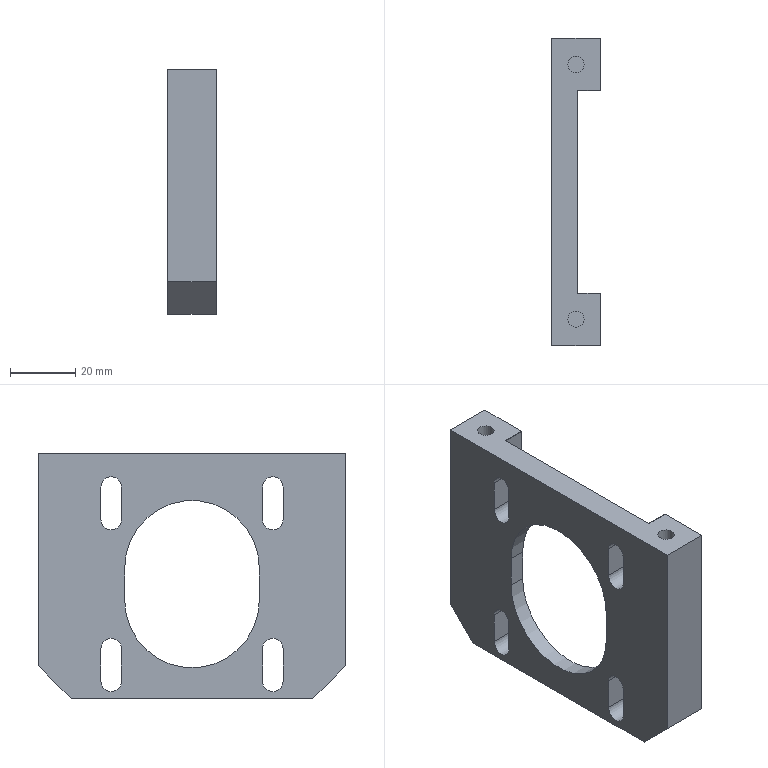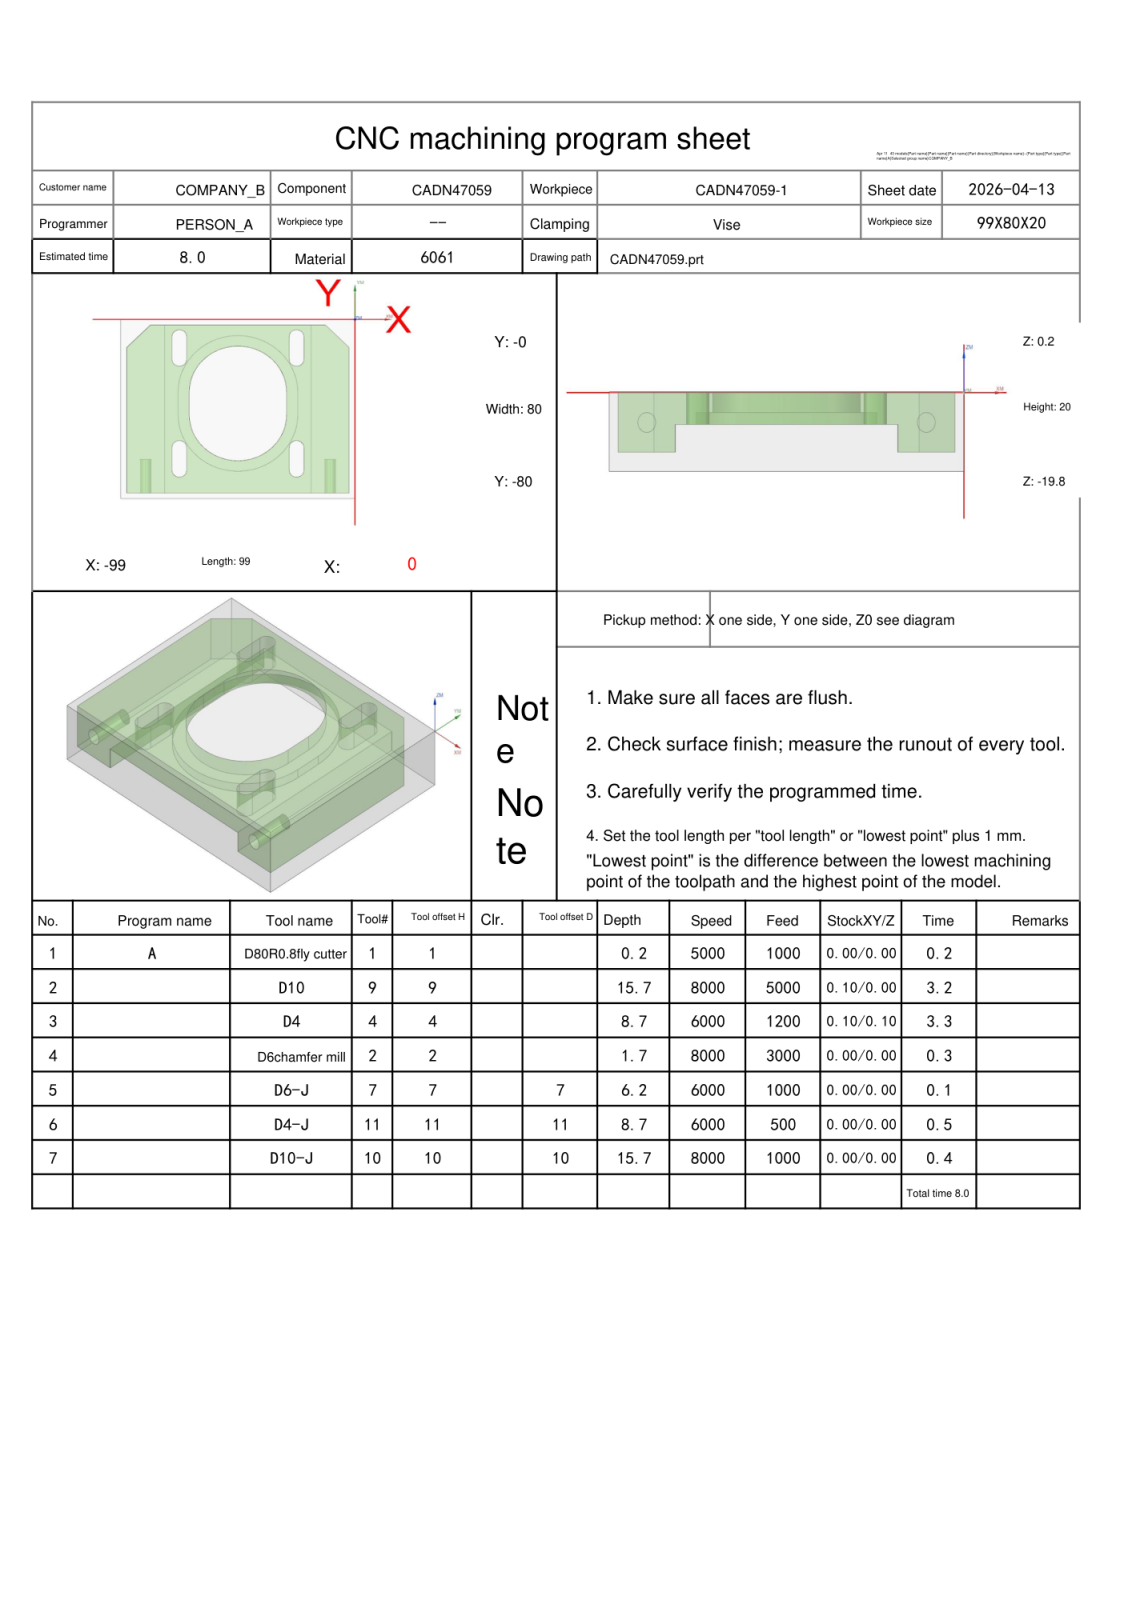NC program | NX | posted by the shop | part box 15 x 94 x 75 mm
Lines 1 to 937 of 2209:
%
O0001
(Machine time: 9.35 MIN)
(===Total Tool:7===)
(T1=D80R0.8 D=80.  R=0.8  D-  H01 Z=0.    )
(T9=D10     D=10.  R=0.   D-  H09 Z=-15.5 )
(T4=D4      D=4.   R=0.   D-  H04 Z=-8.5  )
(T2=D6chamfer mill   D=6.   R=0.   D-  H02 Z=-1.5  )
(T7=D6-J    D=6.   R=0.   D7  H07 Z=-6.   )
(T11=D4-J   D=4.   R=0.   D11 H11 Z=-8.5  )
(T10=D10-J  D=10.  R=0.   D10 H10 Z=-15.5 )
G80 G90 G17 G49 G40
G91 G28 Z0
M01
N1 T01 M06
(D80R0.8  D=80. R=0.8 H=01 ce=0.00 di=0.00)
G00 G90 G54 X-141.5 Y-40. M03 S5000
G43 H01 Z20.
M08
Z2.
G01 Z0.0 F1000.
X-136.5
X37.5
X42.5
Z2.
G00 Z20.
G91 G28 Z0.0
M05
M09
G91 G28 Z0.0
M01
N2 T09 M06
(D10  D=10. R=0. H=09 ce=0.10 di=0.00)
G00 G90 G54 X-49.5 Y-82.6 M03 S8000
G43 H09 Z20.
M08
Z.5
G01 X-96.5 Z.4 F5000.
G02 X-101.6 Y-77.5 Z.383 I0.0 J5.1
G01 Y-12.5 Z.245
G02 X-100.106 Y-8.894 Z.236 I5.1 J0.0
G01 X-90.106 Y1.106 Z.206
G02 X-86.5 Y2.6 Z.198 I3.606 J-3.606
G01 X-12.5 Z.04
G02 X-8.894 Y1.106 Z.032 I0.0 J-5.1
G01 X1.106 Y-8.894 Z.002
G02 X2.6 Y-12.5 Z-.007 I-3.606 J-3.606
G01 Y-77.5 Z-.145
G02 X-2.5 Y-82.6 Z-.162 I-5.1 J0.0
G01 X-96.5 Z-.362
G02 X-101.6 Y-77.5 Z-.379 I0.0 J5.1
G01 Y-12.5 Z-.517
G02 X-100.106 Y-8.894 Z-.526 I5.1 J0.0
G01 X-90.106 Y1.106 Z-.556
G02 X-86.5 Y2.6 Z-.564 I3.606 J-3.606
G01 X-12.5 Z-.722
G02 X-8.894 Y1.106 Z-.73 I0.0 J-5.1
G01 X1.106 Y-8.894 Z-.76
G02 X2.6 Y-12.5 Z-.769 I-3.606 J-3.606
G01 Y-77.5 Z-.907
G02 X-2.5 Y-82.6 Z-.924 I-5.1 J0.0
G01 X-96.5 Z-1.124
G02 X-101.6 Y-77.5 Z-1.141 I0.0 J5.1
G01 Y-12.5 Z-1.279
G02 X-100.106 Y-8.894 Z-1.288 I5.1 J0.0
G01 X-90.106 Y1.106 Z-1.318
G02 X-86.5 Y2.6 Z-1.326 I3.606 J-3.606
G01 X-12.5 Z-1.483
G02 X-8.894 Y1.106 Z-1.492 I0.0 J-5.1
G01 X1.106 Y-8.894 Z-1.522
G02 X2.6 Y-12.5 Z-1.531 I-3.606 J-3.606
G01 Y-77.5 Z-1.669
G02 X-2.5 Y-82.6 Z-1.686 I-5.1 J0.0
G01 X-96.5 Z-1.886
G02 X-101.6 Y-77.5 Z-1.903 I0.0 J5.1
G01 Y-12.5 Z-2.041
G02 X-100.106 Y-8.894 Z-2.049 I5.1 J0.0
G01 X-90.106 Y1.106 Z-2.079
G02 X-86.5 Y2.6 Z-2.088 I3.606 J-3.606
G01 X-12.5 Z-2.245
G02 X-8.894 Y1.106 Z-2.254 I0.0 J-5.1
G01 X1.106 Y-8.894 Z-2.284
G02 X2.6 Y-12.5 Z-2.292 I-3.606 J-3.606
G01 Y-77.5 Z-2.431
G02 X-2.5 Y-82.6 Z-2.448 I-5.1 J0.0
G01 X-96.5 Z-2.648
G02 X-101.6 Y-77.5 Z-2.665 I0.0 J5.1
G01 Y-12.5 Z-2.803
G02 X-100.106 Y-8.894 Z-2.811 I5.1 J0.0
G01 X-90.106 Y1.106 Z-2.841
G02 X-86.5 Y2.6 Z-2.85 I3.606 J-3.606
G01 X-12.5 Z-3.007
G02 X-8.894 Y1.106 Z-3.016 I0.0 J-5.1
G01 X1.106 Y-8.894 Z-3.046
G02 X2.6 Y-12.5 Z-3.054 I-3.606 J-3.606
G01 Y-77.5 Z-3.193
G02 X-2.5 Y-82.6 Z-3.21 I-5.1 J0.0
G01 X-96.5 Z-3.409
G02 X-101.6 Y-77.5 Z-3.426 I0.0 J5.1
G01 Y-12.5 Z-3.565
G02 X-100.106 Y-8.894 Z-3.573 I5.1 J0.0
G01 X-90.106 Y1.106 Z-3.603
G02 X-86.5 Y2.6 Z-3.612 I3.606 J-3.606
G01 X-12.5 Z-3.769
G02 X-8.894 Y1.106 Z-3.778 I0.0 J-5.1
G01 X1.106 Y-8.894 Z-3.808
G02 X2.6 Y-12.5 Z-3.816 I-3.606 J-3.606
G01 Y-77.5 Z-3.954
G02 X-2.5 Y-82.6 Z-3.971 I-5.1 J0.0
G01 X-96.5 Z-4.171
G02 X-101.6 Y-77.5 Z-4.188 I0.0 J5.1
G01 Y-12.5 Z-4.327
G02 X-100.106 Y-8.894 Z-4.335 I5.1 J0.0
G01 X-90.106 Y1.106 Z-4.365
G02 X-86.5 Y2.6 Z-4.374 I3.606 J-3.606
G01 X-12.5 Z-4.531
G02 X-8.894 Y1.106 Z-4.54 I0.0 J-5.1
G01 X1.106 Y-8.894 Z-4.57
G02 X2.6 Y-12.5 Z-4.578 I-3.606 J-3.606
G01 Y-77.5 Z-4.716
G02 X-2.5 Y-82.6 Z-4.733 I-5.1 J0.0
G01 X-96.5 Z-4.933
G02 X-101.6 Y-77.5 Z-4.95 I0.0 J5.1
G01 Y-12.5 Z-5.089
G02 X-100.106 Y-8.894 Z-5.097 I5.1 J0.0
G01 X-90.106 Y1.106 Z-5.127
G02 X-86.5 Y2.6 Z-5.136 I3.606 J-3.606
G01 X-12.5 Z-5.293
G02 X-8.894 Y1.106 Z-5.301 I0.0 J-5.1
G01 X1.106 Y-8.894 Z-5.332
G02 X2.6 Y-12.5 Z-5.34 I-3.606 J-3.606
G01 Y-77.5 Z-5.478
G02 X-2.5 Y-82.6 Z-5.495 I-5.1 J0.0
G01 X-96.5 Z-5.695
G02 X-101.6 Y-77.5 Z-5.712 I0.0 J5.1
G01 Y-12.5 Z-5.85
G02 X-100.106 Y-8.894 Z-5.859 I5.1 J0.0
G01 X-90.106 Y1.106 Z-5.889
G02 X-86.5 Y2.6 Z-5.898 I3.606 J-3.606
G01 X-12.5 Z-6.055
G02 X-8.894 Y1.106 Z-6.063 I0.0 J-5.1
G01 X1.106 Y-8.894 Z-6.093
G02 X2.6 Y-12.5 Z-6.102 I-3.606 J-3.606
G01 Y-77.5 Z-6.24
G02 X-2.5 Y-82.6 Z-6.257 I-5.1 J0.0
G01 X-96.5 Z-6.457
G02 X-101.6 Y-77.5 Z-6.474 I0.0 J5.1
G01 Y-12.5 Z-6.612
G02 X-100.106 Y-8.894 Z-6.621 I5.1 J0.0
G01 X-90.106 Y1.106 Z-6.651
G02 X-86.5 Y2.6 Z-6.659 I3.606 J-3.606
G01 X-12.5 Z-6.817
G02 X-8.894 Y1.106 Z-6.825 I0.0 J-5.1
G01 X1.106 Y-8.894 Z-6.855
G02 X2.6 Y-12.5 Z-6.864 I-3.606 J-3.606
G01 Y-77.5 Z-7.002
G02 X-2.5 Y-82.6 Z-7.019 I-5.1 J0.0
G01 X-96.5 Z-7.219
G02 X-101.6 Y-77.5 Z-7.236 I0.0 J5.1
G01 Y-12.5 Z-7.374
G02 X-100.106 Y-8.894 Z-7.383 I5.1 J0.0
G01 X-90.106 Y1.106 Z-7.413
G02 X-86.5 Y2.6 Z-7.421 I3.606 J-3.606
G01 X-12.5 Z-7.579
G02 X-8.894 Y1.106 Z-7.587 I0.0 J-5.1
G01 X1.106 Y-8.894 Z-7.617
G02 X2.6 Y-12.5 Z-7.626 I-3.606 J-3.606
G01 Y-77.5 Z-7.764
G02 X-2.5 Y-82.6 Z-7.781 I-5.1 J0.0
G01 X-96.5 Z-7.981
G02 X-101.6 Y-77.5 Z-7.998 I0.0 J5.1
G01 Y-12.5 Z-8.136
G02 X-100.106 Y-8.894 Z-8.145 I5.1 J0.0
G01 X-90.106 Y1.106 Z-8.175
G02 X-86.5 Y2.6 Z-8.183 I3.606 J-3.606
G01 X-12.5 Z-8.341
G02 X-8.894 Y1.106 Z-8.349 I0.0 J-5.1
G01 X1.106 Y-8.894 Z-8.379
G02 X2.6 Y-12.5 Z-8.388 I-3.606 J-3.606
G01 Y-77.5 Z-8.526
G02 X-2.5 Y-82.6 Z-8.543 I-5.1 J0.0
G01 X-96.5 Z-8.743
G02 X-101.6 Y-77.5 Z-8.76 I0.0 J5.1
G01 Y-12.5 Z-8.898
G02 X-100.106 Y-8.894 Z-8.907 I5.1 J0.0
G01 X-90.106 Y1.106 Z-8.937
G02 X-86.5 Y2.6 Z-8.945 I3.606 J-3.606
G01 X-12.5 Z-9.102
G02 X-8.894 Y1.106 Z-9.111 I0.0 J-5.1
G01 X1.106 Y-8.894 Z-9.141
G02 X2.6 Y-12.5 Z-9.15 I-3.606 J-3.606
G01 Y-77.5 Z-9.288
G02 X-2.5 Y-82.6 Z-9.305 I-5.1 J0.0
G01 X-96.5 Z-9.505
G02 X-101.6 Y-77.5 Z-9.522 I0.0 J5.1
G01 Y-12.5 Z-9.66
G02 X-100.106 Y-8.894 Z-9.668 I5.1 J0.0
G01 X-90.106 Y1.106 Z-9.699
G02 X-86.5 Y2.6 Z-9.707 I3.606 J-3.606
G01 X-12.5 Z-9.864
G02 X-8.894 Y1.106 Z-9.873 I0.0 J-5.1
G01 X1.106 Y-8.894 Z-9.903
G02 X2.6 Y-12.5 Z-9.911 I-3.606 J-3.606
G01 Y-77.5 Z-10.05
G02 X-2.5 Y-82.6 Z-10.067 I-5.1 J0.0
G01 X-96.5 Z-10.267
G02 X-101.6 Y-77.5 Z-10.284 I0.0 J5.1
G01 Y-12.5 Z-10.422
G02 X-100.106 Y-8.894 Z-10.43 I5.1 J0.0
G01 X-90.106 Y1.106 Z-10.46
G02 X-86.5 Y2.6 Z-10.469 I3.606 J-3.606
G01 X-12.5 Z-10.626
G02 X-8.894 Y1.106 Z-10.635 I0.0 J-5.1
G01 X1.106 Y-8.894 Z-10.665
G02 X2.6 Y-12.5 Z-10.673 I-3.606 J-3.606
G01 Y-77.5 Z-10.812
G02 X-2.5 Y-82.6 Z-10.829 I-5.1 J0.0
G01 X-96.5 Z-11.029
G02 X-101.6 Y-77.5 Z-11.046 I0.0 J5.1
G01 Y-12.5 Z-11.184
G02 X-100.106 Y-8.894 Z-11.192 I5.1 J0.0
G01 X-90.106 Y1.106 Z-11.222
G02 X-86.5 Y2.6 Z-11.231 I3.606 J-3.606
G01 X-12.5 Z-11.388
G02 X-8.894 Y1.106 Z-11.397 I0.0 J-5.1
G01 X1.106 Y-8.894 Z-11.427
G02 X2.6 Y-12.5 Z-11.435 I-3.606 J-3.606
G01 Y-77.5 Z-11.574
G02 X-2.5 Y-82.6 Z-11.591 I-5.1 J0.0
G01 X-96.5 Z-11.79
G02 X-101.6 Y-77.5 Z-11.807 I0.0 J5.1
G01 Y-12.5 Z-11.946
G02 X-100.106 Y-8.894 Z-11.954 I5.1 J0.0
G01 X-90.106 Y1.106 Z-11.984
G02 X-86.5 Y2.6 Z-11.993 I3.606 J-3.606
G01 X-12.5 Z-12.15
G02 X-8.894 Y1.106 Z-12.159 I0.0 J-5.1
G01 X1.106 Y-8.894 Z-12.189
G02 X2.6 Y-12.5 Z-12.197 I-3.606 J-3.606
G01 Y-77.5 Z-12.335
G02 X-2.5 Y-82.6 Z-12.352 I-5.1 J0.0
G01 X-96.5 Z-12.552
G02 X-101.6 Y-77.5 Z-12.569 I0.0 J5.1
G01 Y-12.5 Z-12.708
G02 X-100.106 Y-8.894 Z-12.716 I5.1 J0.0
G01 X-90.106 Y1.106 Z-12.746
G02 X-86.5 Y2.6 Z-12.755 I3.606 J-3.606
G01 X-12.5 Z-12.912
G02 X-8.894 Y1.106 Z-12.921 I0.0 J-5.1
G01 X1.106 Y-8.894 Z-12.951
G02 X2.6 Y-12.5 Z-12.959 I-3.606 J-3.606
G01 Y-77.5 Z-13.097
G02 X-2.5 Y-82.6 Z-13.114 I-5.1 J0.0
G01 X-96.5 Z-13.314
G02 X-101.6 Y-77.5 Z-13.331 I0.0 J5.1
G01 Y-12.5 Z-13.469
G02 X-100.106 Y-8.894 Z-13.478 I5.1 J0.0
G01 X-90.106 Y1.106 Z-13.508
G02 X-86.5 Y2.6 Z-13.517 I3.606 J-3.606
G01 X-12.5 Z-13.674
G02 X-8.894 Y1.106 Z-13.682 I0.0 J-5.1
G01 X1.106 Y-8.894 Z-13.712
G02 X2.6 Y-12.5 Z-13.721 I-3.606 J-3.606
G01 Y-77.5 Z-13.859
G02 X-2.5 Y-82.6 Z-13.876 I-5.1 J0.0
G01 X-96.5 Z-14.076
G02 X-101.6 Y-77.5 Z-14.093 I0.0 J5.1
G01 Y-12.5 Z-14.231
G02 X-100.106 Y-8.894 Z-14.24 I5.1 J0.0
G01 X-90.106 Y1.106 Z-14.27
G02 X-86.5 Y2.6 Z-14.278 I3.606 J-3.606
G01 X-12.5 Z-14.436
G02 X-8.894 Y1.106 Z-14.444 I0.0 J-5.1
G01 X1.106 Y-8.894 Z-14.474
G02 X2.6 Y-12.5 Z-14.483 I-3.606 J-3.606
G01 Y-77.5 Z-14.621
G02 X-2.5 Y-82.6 Z-14.638 I-5.1 J0.0
G01 X-96.5 Z-14.838
G02 X-101.6 Y-77.5 Z-14.855 I0.0 J5.1
G01 Y-12.5 Z-14.993
G02 X-100.106 Y-8.894 Z-15.002 I5.1 J0.0
G01 X-90.106 Y1.106 Z-15.032
G02 X-86.5 Y2.6 Z-15.04 I3.606 J-3.606
G01 X-12.5 Z-15.198
G02 X-8.894 Y1.106 Z-15.206 I0.0 J-5.1
G01 X1.106 Y-8.894 Z-15.236
G02 X2.6 Y-12.5 Z-15.245 I-3.606 J-3.606
G01 Y-77.5 Z-15.383
G02 X-2.5 Y-82.6 Z-15.4 I-5.1 J0.0
G01 X-49.5 Z-15.5
X-96.5
G02 X-101.6 Y-77.5 I0.0 J5.1
G01 Y-12.5
G02 X-100.106 Y-8.894 I5.1 J0.0
G01 X-90.106 Y1.106
G02 X-86.5 Y2.6 I3.606 J-3.606
G01 X-12.5
G02 X-8.894 Y1.106 I0.0 J-5.1
G01 X1.106 Y-8.894
G02 X2.6 Y-12.5 I-3.606 J-3.606
G01 Y-77.5
G02 X-2.5 Y-82.6 I-5.1 J0.0
G01 X-49.5
X-50.
Z-14.5
G00 Z20.
G00 G90 X-55.245 Y-38.997 M03 S8000
Z10.2
Z1.5
G02 X-55.245 Y-38.997 Z.018 I-4.255 J1.466 F3000.
X-63.182 Y-40.118 Z-.5 I-4.255 J1.466
G01 X-65. Y-37.531
Y-32.5
G02 X-49.5 Y-17. I15.5 J0.0
X-34. Y-32.5 I0.0 J-15.5
G01 Y-42.5
G02 X-49.5 Y-58. I-15.5 J0.0
X-64.999 Y-42.703 I0.0 J15.5
G01 X-65. Y-37.531
Y-33.25
G02 X-64.318 Y-32.303 I1. J0.0
G01 X-58.118 Y-30.225
G03 X-57.496 Y-29.616 I-.318 J.948
G02 X-49.5 Y-24. I7.996 J-2.884
X-41. Y-32.5 I0.0 J-8.5
G01 Y-42.5
G02 X-49.5 Y-51. I-8.5 J0.0
X-57.999 Y-42.649 I0.0 J8.5
G01 X-58. Y-37.531
Y-35.733
G02 X-57.34 Y-34.793 I1. J0.0
G01 X-51.547 Y-32.698
G03 X-50.932 Y-32.055 I-.34 J.94
G02 X-49.5 Y-31. I1.432 J-.445
X-48. Y-32.5 I0.0 J-1.5
G01 Y-42.5
G02 X-49.5 Y-44. I-1.5 J0.0
X-50.999 Y-42.562 I0.0 J1.5
G01 X-51. Y-37.625
Y-32.531
Y-32.5
G02 X-50.927 Y-32.039 I1.5 J0.0
G03 X-50.588 Y-29.886 I-6.661 J2.153
X-55.435 Y-23.225 I-7. J0.0
G01 Z.7
G00 Z3.
G01 X-55.245 Y-38.997 F6000.
G00 Z1.
G02 X-55.245 Y-38.997 Z-.482 I-4.255 J1.466 F3000.
X-63.182 Y-40.118 Z-1. I-4.255 J1.466
G01 X-65. Y-37.531
Y-32.5
G02 X-49.5 Y-17. I15.5 J0.0
X-34. Y-32.5 I0.0 J-15.5
G01 Y-42.5
G02 X-49.5 Y-58. I-15.5 J0.0
X-64.999 Y-42.703 I0.0 J15.5
G01 X-65. Y-37.531
Y-32.531
G02 X-64.221 Y-31.556 I1. J0.0
G01 X-58.193 Y-30.19
G03 X-57.476 Y-29.561 I-.221 J.975
G02 X-49.5 Y-24. I7.976 J-2.939
X-41. Y-32.5 I0.0 J-8.5
G01 Y-42.5
G02 X-49.5 Y-51. I-8.5 J0.0
X-57.999 Y-42.649 I0.0 J8.5
G01 X-58. Y-37.531
Y-35.655
G02 X-57.44 Y-34.757 I1. J0.0
G01 X-50.515 Y-31.365
X-50.373 Y-31.28
G02 X-49.5 Y-31. I.873 J-1.22
X-48. Y-32.5 I0.0 J-1.5
G01 Y-42.5
G02 X-49.5 Y-44. I-1.5 J0.0
X-50.999 Y-42.562 I0.0 J1.5
G01 X-51. Y-37.625
Y-32.531
Y-32.5
G02 X-50.927 Y-32.039 I1.5 J0.0
G03 X-50.588 Y-29.886 I-6.661 J2.153
X-55.435 Y-23.225 I-7. J0.0
G01 Z.2
G00 Z2.5
G01 X-55.245 Y-38.997 F6000.
G00 Z.5
G02 X-55.245 Y-38.997 Z-.982 I-4.255 J1.466 F3000.
X-63.182 Y-40.118 Z-1.5 I-4.255 J1.466
G01 X-65. Y-37.531
Y-32.5
G02 X-49.5 Y-17. I15.5 J0.0
X-34. Y-32.5 I0.0 J-15.5
G01 Y-42.5
G02 X-49.5 Y-58. I-15.5 J0.0
X-64.999 Y-42.703 I0.0 J15.5
G01 X-65. Y-37.531
Y-32.531
G02 X-64.221 Y-31.556 I1. J0.0
G01 X-58.193 Y-30.19
G03 X-57.476 Y-29.561 I-.221 J.975
G02 X-49.5 Y-24. I7.976 J-2.939
X-41. Y-32.5 I0.0 J-8.5
G01 Y-42.5
G02 X-49.5 Y-51. I-8.5 J0.0
X-57.999 Y-42.649 I0.0 J8.5
G01 X-58. Y-37.531
Y-35.733
G02 X-57.34 Y-34.793 I1. J0.0
G01 X-51.547 Y-32.698
G03 X-50.932 Y-32.055 I-.34 J.94
G02 X-49.5 Y-31. I1.432 J-.445
X-48. Y-32.5 I0.0 J-1.5
G01 Y-42.5
G02 X-49.5 Y-44. I-1.5 J0.0
X-50.999 Y-42.562 I0.0 J1.5
G01 X-51. Y-37.625
Y-32.531
Y-32.5
G02 X-50.927 Y-32.039 I1.5 J0.0
G03 X-50.588 Y-29.886 I-6.661 J2.153
X-55.435 Y-23.225 I-7. J0.0
G01 Z-.3
G00 Z2.
G01 X-55.245 Y-38.997 F6000.
G00 Z0.0
G02 X-55.245 Y-38.997 Z-1.482 I-4.255 J1.466 F3000.
X-63.182 Y-40.118 Z-2. I-4.255 J1.466
G01 X-65. Y-37.531
Y-32.5
G02 X-49.5 Y-17. I15.5 J0.0
X-34. Y-32.5 I0.0 J-15.5
G01 Y-42.5
G02 X-49.5 Y-58. I-15.5 J0.0
X-64.999 Y-42.703 I0.0 J15.5
G01 X-65. Y-37.531
Y-32.531
G02 X-64.221 Y-31.556 I1. J0.0
G01 X-58.193 Y-30.19
G03 X-57.476 Y-29.561 I-.221 J.975
G02 X-49.5 Y-24. I7.976 J-2.939
X-41. Y-32.5 I0.0 J-8.5
G01 Y-42.5
G02 X-49.5 Y-51. I-8.5 J0.0
X-57.999 Y-42.649 I0.0 J8.5
G01 X-58. Y-37.531
Y-35.733
G02 X-57.34 Y-34.793 I1. J0.0
G01 X-51.547 Y-32.698
G03 X-50.932 Y-32.055 I-.34 J.94
G02 X-49.5 Y-31. I1.432 J-.445
X-48. Y-32.5 I0.0 J-1.5
G01 Y-42.5
G02 X-49.5 Y-44. I-1.5 J0.0
X-50.999 Y-42.562 I0.0 J1.5
G01 X-51. Y-37.625
Y-32.531
Y-32.5
G02 X-50.927 Y-32.039 I1.5 J0.0
G03 X-50.588 Y-29.886 I-6.661 J2.153
X-55.435 Y-23.225 I-7. J0.0
G01 Z-.8
G00 Z1.5
G01 X-55.245 Y-38.997 F6000.
G00 Z-.5
G02 X-55.245 Y-38.997 Z-1.982 I-4.255 J1.466 F3000.
X-63.182 Y-40.118 Z-2.5 I-4.255 J1.466
G01 X-65. Y-37.531
Y-32.5
G02 X-49.5 Y-17. I15.5 J0.0
X-34. Y-32.5 I0.0 J-15.5
G01 Y-42.5
G02 X-49.5 Y-58. I-15.5 J0.0
X-64.999 Y-42.703 I0.0 J15.5
G01 X-65. Y-37.531
Y-32.531
G02 X-64.221 Y-31.556 I1. J0.0
G01 X-58.193 Y-30.19
G03 X-57.476 Y-29.561 I-.221 J.975
G02 X-49.5 Y-24. I7.976 J-2.939
X-41. Y-32.5 I0.0 J-8.5
G01 Y-42.5
G02 X-49.5 Y-51. I-8.5 J0.0
X-57.999 Y-42.649 I0.0 J8.5
G01 X-58. Y-37.531
Y-35.733
G02 X-57.34 Y-34.793 I1. J0.0
G01 X-51.547 Y-32.698
G03 X-50.932 Y-32.055 I-.34 J.94
G02 X-49.5 Y-31. I1.432 J-.445
X-48. Y-32.5 I0.0 J-1.5
G01 Y-42.5
G02 X-49.5 Y-44. I-1.5 J0.0
X-50.999 Y-42.562 I0.0 J1.5
G01 X-51. Y-37.625
Y-32.531
Y-32.5
G02 X-50.927 Y-32.039 I1.5 J0.0
G03 X-50.588 Y-29.886 I-6.661 J2.153
X-55.435 Y-23.225 I-7. J0.0
G01 Z-1.3
G00 Z1.
G01 X-55.245 Y-38.997 F6000.
G00 Z-1.
G02 X-55.245 Y-38.997 Z-2.482 I-4.255 J1.466 F3000.
X-63.182 Y-40.118 Z-3. I-4.255 J1.466
G01 X-65. Y-37.531
Y-32.5
G02 X-49.5 Y-17. I15.5 J0.0
X-34. Y-32.5 I0.0 J-15.5
G01 Y-42.5
G02 X-49.5 Y-58. I-15.5 J0.0
X-64.999 Y-42.703 I0.0 J15.5
G01 X-65. Y-37.531
Y-32.531
G02 X-64.221 Y-31.556 I1. J0.0
G01 X-58.193 Y-30.19
G03 X-57.476 Y-29.561 I-.221 J.975
G02 X-49.5 Y-24. I7.976 J-2.939
X-41. Y-32.5 I0.0 J-8.5
G01 Y-42.5
G02 X-49.5 Y-51. I-8.5 J0.0
X-57.999 Y-42.649 I0.0 J8.5
G01 X-58. Y-37.531
Y-35.733
G02 X-57.34 Y-34.793 I1. J0.0
G01 X-51.547 Y-32.698
G03 X-50.932 Y-32.055 I-.34 J.94
G02 X-49.5 Y-31. I1.432 J-.445
X-48. Y-32.5 I0.0 J-1.5
G01 Y-42.5
G02 X-49.5 Y-44. I-1.5 J0.0
X-50.999 Y-42.562 I0.0 J1.5
G01 X-51. Y-37.625
Y-32.531
Y-32.5
G02 X-50.927 Y-32.039 I1.5 J0.0
G03 X-50.588 Y-29.886 I-6.661 J2.153
X-55.435 Y-23.225 I-7. J0.0
G01 Z-1.8
G00 Z.5
G01 X-55.245 Y-38.997 F6000.
G00 Z-1.5
G02 X-55.245 Y-38.997 Z-2.982 I-4.255 J1.466 F3000.
X-63.182 Y-40.118 Z-3.5 I-4.255 J1.466
G01 X-65. Y-37.531
Y-32.5
G02 X-49.5 Y-17. I15.5 J0.0
X-34. Y-32.5 I0.0 J-15.5
G01 Y-42.5
G02 X-49.5 Y-58. I-15.5 J0.0
X-64.999 Y-42.703 I0.0 J15.5
G01 X-65. Y-37.531
Y-33.25
G02 X-64.318 Y-32.303 I1. J0.0
G01 X-58.118 Y-30.225
G03 X-57.496 Y-29.616 I-.318 J.948
G02 X-49.5 Y-24. I7.996 J-2.884
X-41. Y-32.5 I0.0 J-8.5
G01 Y-42.5
G02 X-49.5 Y-51. I-8.5 J0.0
X-57.999 Y-42.649 I0.0 J8.5
G01 X-58. Y-37.531
Y-35.733
G02 X-57.34 Y-34.793 I1. J0.0
G01 X-51.547 Y-32.698
G03 X-50.932 Y-32.055 I-.34 J.94
G02 X-49.5 Y-31. I1.432 J-.445
X-48. Y-32.5 I0.0 J-1.5
G01 Y-42.5
G02 X-49.5 Y-44. I-1.5 J0.0
X-50.999 Y-42.562 I0.0 J1.5
G01 X-51. Y-37.625
Y-32.531
Y-32.5
G02 X-50.927 Y-32.039 I1.5 J0.0
G03 X-50.588 Y-29.886 I-6.661 J2.153
X-55.435 Y-23.225 I-7. J0.0
G01 Z-2.3
G00 Z0.0
G01 X-55.245 Y-38.997 F6000.
G00 Z-2.
G02 X-55.245 Y-38.997 Z-3.482 I-4.255 J1.466 F3000.
X-63.182 Y-40.118 Z-4. I-4.255 J1.466
G01 X-65. Y-37.531
Y-32.5
G02 X-49.5 Y-17. I15.5 J0.0
X-34. Y-32.5 I0.0 J-15.5
G01 Y-42.5
G02 X-49.5 Y-58. I-15.5 J0.0
X-64.999 Y-42.703 I0.0 J15.5
G01 X-65. Y-37.531
Y-32.531
G02 X-64.221 Y-31.556 I1. J0.0
G01 X-58.193 Y-30.19
G03 X-57.476 Y-29.561 I-.221 J.975
G02 X-49.5 Y-24. I7.976 J-2.939
X-41. Y-32.5 I0.0 J-8.5
G01 Y-42.5
G02 X-49.5 Y-51. I-8.5 J0.0
X-57.999 Y-42.649 I0.0 J8.5
G01 X-58. Y-37.531
Y-35.733
G02 X-57.34 Y-34.793 I1. J0.0
G01 X-51.547 Y-32.698
G03 X-50.932 Y-32.055 I-.34 J.94
G02 X-49.5 Y-31. I1.432 J-.445
X-48. Y-32.5 I0.0 J-1.5
G01 Y-42.5
G02 X-49.5 Y-44. I-1.5 J0.0
X-50.999 Y-42.562 I0.0 J1.5
G01 X-51. Y-37.626
Y-32.531
Y-32.5
G02 X-50.927 Y-32.039 I1.5 J0.0
G03 X-50.588 Y-29.886 I-6.661 J2.153
X-55.435 Y-23.225 I-7. J0.0
G01 Z-2.8
G00 Z-.5
G01 X-55.245 Y-38.997 F6000.
G00 Z-2.5
G02 X-55.245 Y-38.997 Z-3.982 I-4.255 J1.466 F3000.
X-63.182 Y-40.118 Z-4.5 I-4.255 J1.466
G01 X-65. Y-37.531
Y-32.5
G02 X-49.5 Y-17. I15.5 J0.0
X-34. Y-32.5 I0.0 J-15.5
G01 Y-42.5
G02 X-49.5 Y-58. I-15.5 J0.0
X-64.999 Y-42.703 I0.0 J15.5
G01 X-65. Y-37.531
Y-33.25
G02 X-64.318 Y-32.303 I1. J0.0
G01 X-58.118 Y-30.225
G03 X-57.496 Y-29.616 I-.318 J.948
G02 X-49.5 Y-24. I7.996 J-2.884
X-41. Y-32.5 I0.0 J-8.5
G01 Y-42.5
G02 X-49.5 Y-51. I-8.5 J0.0
X-57.999 Y-42.649 I0.0 J8.5
G01 X-58. Y-37.531
Y-35.733
G02 X-57.34 Y-34.793 I1. J0.0
G01 X-51.547 Y-32.698
G03 X-50.932 Y-32.055 I-.34 J.94
G02 X-49.5 Y-31. I1.432 J-.445
X-48. Y-32.5 I0.0 J-1.5
G01 Y-42.5
G02 X-49.5 Y-44. I-1.5 J0.0
X-50.998 Y-42.577 I0.0 J1.5
G01 X-51. Y-32.53
Y-32.5
G02 X-50.927 Y-32.037 I1.5 J0.0
G03 X-50.586 Y-29.878 I-6.659 J2.159
X-55.427 Y-23.22 I-7. J0.0
G01 Z-3.3
G00 Z-1.
G01 X-55.245 Y-38.997 F6000.
G00 Z-3.
G02 X-55.245 Y-38.997 Z-4.482 I-4.255 J1.466 F3000.
X-63.182 Y-40.118 Z-5. I-4.255 J1.466
G01 X-65. Y-37.531
Y-32.5
G02 X-49.5 Y-17. I15.5 J0.0
X-34. Y-32.5 I0.0 J-15.5
G01 Y-42.5
G02 X-49.5 Y-58. I-15.5 J0.0
X-64.999 Y-42.703 I0.0 J15.5
G01 X-65. Y-37.531
Y-32.531
G02 X-64.221 Y-31.556 I1. J0.0
G01 X-58.193 Y-30.19
G03 X-57.476 Y-29.561 I-.221 J.975
G02 X-49.5 Y-24. I7.976 J-2.939
X-41. Y-32.5 I0.0 J-8.5
G01 Y-42.5
G02 X-49.5 Y-51. I-8.5 J0.0
X-57.999 Y-42.649 I0.0 J8.5
G01 X-58. Y-37.531
Y-35.733
G02 X-57.34 Y-34.793 I1. J0.0
G01 X-51.547 Y-32.698
G03 X-50.932 Y-32.055 I-.34 J.94
G02 X-49.5 Y-31. I1.432 J-.445
X-48. Y-32.5 I0.0 J-1.5
G01 Y-42.5
G02 X-49.5 Y-44. I-1.5 J0.0
X-50.999 Y-42.562 I0.0 J1.5
G01 X-51. Y-37.626
Y-32.531
Y-32.5
G02 X-50.927 Y-32.039 I1.5 J0.0
G03 X-50.588 Y-29.886 I-6.661 J2.153
X-55.435 Y-23.225 I-7. J0.0
G01 Z-3.8
G00 Z-1.5
G01 X-55.245 Y-38.997 F6000.
G00 Z-3.5
G02 X-55.245 Y-38.997 Z-4.982 I-4.255 J1.466 F3000.
X-63.182 Y-40.118 Z-5.5 I-4.255 J1.466
G01 X-65. Y-37.531
Y-32.5
G02 X-49.5 Y-17. I15.5 J0.0
X-34. Y-32.5 I0.0 J-15.5
G01 Y-42.5
G02 X-49.5 Y-58. I-15.5 J0.0
X-64.999 Y-42.703 I0.0 J15.5
G01 X-65. Y-37.531
Y-32.531
G02 X-64.221 Y-31.556 I1. J0.0
G01 X-58.193 Y-30.19
G03 X-57.476 Y-29.561 I-.221 J.975
G02 X-49.5 Y-24. I7.976 J-2.939
X-41. Y-32.5 I0.0 J-8.5
G01 Y-42.5
G02 X-49.5 Y-51. I-8.5 J0.0
X-57.999 Y-42.649 I0.0 J8.5
G01 X-58. Y-37.531
Y-35.733
G02 X-57.34 Y-34.793 I1. J0.0
G01 X-51.547 Y-32.698
G03 X-50.932 Y-32.055 I-.34 J.94
G02 X-49.5 Y-31. I1.432 J-.445
X-48. Y-32.5 I0.0 J-1.5
G01 Y-42.5
G02 X-49.5 Y-44. I-1.5 J0.0
X-50.999 Y-42.562 I0.0 J1.5
G01 X-51. Y-37.626
Y-32.531
Y-32.5
G02 X-50.927 Y-32.039 I1.5 J0.0
G03 X-50.588 Y-29.886 I-6.661 J2.153
X-55.435 Y-23.225 I-7. J0.0
G01 Z-4.3
G00 Z-2.
G01 X-55.245 Y-38.997 F6000.
G00 Z-4.
G02 X-55.245 Y-38.997 Z-5.482 I-4.255 J1.466 F3000.
X-63.182 Y-40.118 Z-6. I-4.255 J1.466
G01 X-65. Y-37.531
Y-32.5
G02 X-49.5 Y-17. I15.5 J0.0
X-34. Y-32.5 I0.0 J-15.5
G01 Y-42.5
G02 X-49.5 Y-58. I-15.5 J0.0
X-64.999 Y-42.703 I0.0 J15.5
G01 X-65. Y-37.531
Y-32.531
G02 X-64.221 Y-31.556 I1. J0.0
G01 X-58.193 Y-30.19
G03 X-57.476 Y-29.561 I-.221 J.975
G02 X-49.5 Y-24. I7.976 J-2.939
X-41. Y-32.5 I0.0 J-8.5
G01 Y-42.5
G02 X-49.5 Y-51. I-8.5 J0.0
X-57.999 Y-42.649 I0.0 J8.5
G01 X-58. Y-37.531
Y-35.733
G02 X-57.34 Y-34.793 I1. J0.0
G01 X-51.547 Y-32.698
G03 X-50.932 Y-32.055 I-.34 J.94
G02 X-49.5 Y-31. I1.432 J-.445
X-48. Y-32.5 I0.0 J-1.5
G01 Y-42.5
G02 X-49.5 Y-44. I-1.5 J0.0
X-50.999 Y-42.562 I0.0 J1.5
G01 X-51. Y-37.626
Y-32.531
Y-32.5
G02 X-50.927 Y-32.039 I1.5 J0.0
G03 X-50.588 Y-29.886 I-6.661 J2.153
X-55.435 Y-23.225 I-7. J0.0
G01 Z-4.8
G00 Z-2.5
G01 X-55.245 Y-38.997 F6000.
G00 Z-4.5
G02 X-55.245 Y-38.997 Z-5.982 I-4.255 J1.466 F3000.
X-63.182 Y-40.118 Z-6.5 I-4.255 J1.466
G01 X-65. Y-37.531
Y-32.5
G02 X-49.5 Y-17. I15.5 J0.0
X-34. Y-32.5 I0.0 J-15.5
G01 Y-42.5
G02 X-49.5 Y-58. I-15.5 J0.0
X-64.999 Y-42.703 I0.0 J15.5
G01 X-65. Y-37.531
Y-32.531
G02 X-64.221 Y-31.556 I1. J0.0
G01 X-58.193 Y-30.19
G03 X-57.476 Y-29.561 I-.221 J.975
G02 X-49.5 Y-24. I7.976 J-2.939
X-41. Y-32.5 I0.0 J-8.5
G01 Y-42.5
G02 X-49.5 Y-51. I-8.5 J0.0
X-57.999 Y-42.649 I0.0 J8.5
G01 X-58. Y-37.531
Y-35.733
G02 X-57.34 Y-34.793 I1. J0.0
G01 X-51.547 Y-32.698
G03 X-50.932 Y-32.055 I-.34 J.94
G02 X-49.5 Y-31. I1.432 J-.445
X-48. Y-32.5 I0.0 J-1.5
G01 Y-42.5
G02 X-49.5 Y-44. I-1.5 J0.0
X-50.999 Y-42.562 I0.0 J1.5
G01 X-51. Y-37.626
Y-32.531
Y-32.5
G02 X-50.927 Y-32.039 I1.5 J0.0
G03 X-50.588 Y-29.886 I-6.661 J2.153
X-55.435 Y-23.225 I-7. J0.0
G01 Z-5.3
G00 Z-3.
G01 X-55.245 Y-38.997 F6000.
G00 Z-5.
G02 X-55.245 Y-38.997 Z-6.482 I-4.255 J1.466 F3000.
X-63.182 Y-40.118 Z-7. I-4.255 J1.466
G01 X-65. Y-37.531
Y-32.5
G02 X-49.5 Y-17. I15.5 J0.0
X-34. Y-32.5 I0.0 J-15.5
G01 Y-42.5
G02 X-49.5 Y-58. I-15.5 J0.0
X-64.999 Y-42.703 I0.0 J15.5
G01 X-65. Y-37.531
Y-32.531
G02 X-64.221 Y-31.556 I1. J0.0
G01 X-58.193 Y-30.19
G03 X-57.476 Y-29.561 I-.221 J.975
G02 X-49.5 Y-24. I7.976 J-2.939
X-41. Y-32.5 I0.0 J-8.5
G01 Y-42.5
G02 X-49.5 Y-51. I-8.5 J0.0
X-57.999 Y-42.649 I0.0 J8.5
G01 X-58. Y-37.531
Y-35.733
G02 X-57.34 Y-34.793 I1. J0.0
G01 X-51.547 Y-32.698
G03 X-50.932 Y-32.055 I-.34 J.94
G02 X-49.5 Y-31. I1.432 J-.445
X-48. Y-32.5 I0.0 J-1.5
G01 Y-42.5
G02 X-49.5 Y-44. I-1.5 J0.0
X-50.999 Y-42.562 I0.0 J1.5
G01 X-51. Y-37.626
Y-32.531
Y-32.5
G02 X-50.927 Y-32.039 I1.5 J0.0
G03 X-50.588 Y-29.886 I-6.661 J2.153
X-55.435 Y-23.225 I-7. J0.0
G01 Z-5.8
G00 Z-3.5
G01 X-55.245 Y-38.997 F6000.
G00 Z-5.5
G02 X-55.245 Y-38.997 Z-6.982 I-4.255 J1.466 F3000.
X-63.182 Y-40.118 Z-7.5 I-4.255 J1.466
G01 X-65. Y-37.531
Y-32.5
G02 X-49.5 Y-17. I15.5 J0.0
X-34. Y-32.5 I0.0 J-15.5
G01 Y-42.5
G02 X-49.5 Y-58. I-15.5 J0.0
X-64.999 Y-42.703 I0.0 J15.5
G01 X-65. Y-37.531
Y-32.531
G02 X-64.221 Y-31.556 I1. J0.0
G01 X-58.193 Y-30.19
G03 X-57.476 Y-29.561 I-.221 J.975
G02 X-49.5 Y-24. I7.976 J-2.939
X-41. Y-32.5 I0.0 J-8.5
G01 Y-42.5
G02 X-49.5 Y-51. I-8.5 J0.0
X-57.999 Y-42.649 I0.0 J8.5
G01 X-58. Y-37.531
Y-35.733
G02 X-57.34 Y-34.793 I1. J0.0
G01 X-51.547 Y-32.698
G03 X-50.932 Y-32.055 I-.34 J.94
G02 X-49.5 Y-31. I1.432 J-.445
X-48. Y-32.5 I0.0 J-1.5
G01 Y-42.5
G02 X-49.5 Y-44. I-1.5 J0.0
X-50.999 Y-42.562 I0.0 J1.5
G01 X-51. Y-37.626
Y-32.531
Y-32.5
G02 X-50.927 Y-32.039 I1.5 J0.0
G03 X-50.588 Y-29.886 I-6.661 J2.153
X-55.435 Y-23.225 I-7. J0.0
G01 Z-6.3
G00 Z-4.
G01 X-55.245 Y-38.997 F6000.
G00 Z-6.
G02 X-55.245 Y-38.997 Z-7.482 I-4.255 J1.466 F3000.
X-63.182 Y-40.118 Z-8. I-4.255 J1.466
G01 X-65. Y-37.531
Y-32.5
G02 X-49.5 Y-17. I15.5 J0.0
X-34. Y-32.5 I0.0 J-15.5
G01 Y-42.5
G02 X-49.5 Y-58. I-15.5 J0.0
X-64.999 Y-42.703 I0.0 J15.5
G01 X-65. Y-37.531
Y-32.531
G02 X-64.221 Y-31.556 I1. J0.0
G01 X-58.193 Y-30.19
G03 X-57.476 Y-29.561 I-.221 J.975
G02 X-49.5 Y-24. I7.976 J-2.939
X-41. Y-32.5 I0.0 J-8.5
G01 Y-42.5
G02 X-49.5 Y-51. I-8.5 J0.0
X-57.999 Y-42.649 I0.0 J8.5
G01 X-58. Y-37.531
Y-35.733
G02 X-57.34 Y-34.793 I1. J0.0
G01 X-51.547 Y-32.698
G03 X-50.932 Y-32.055 I-.34 J.94
G02 X-49.5 Y-31. I1.432 J-.445
X-48. Y-32.5 I0.0 J-1.5
G01 Y-42.5
G02 X-49.5 Y-44. I-1.5 J0.0
X-50.999 Y-42.562 I0.0 J1.5
G01 X-51. Y-37.627
Y-32.531
Y-32.5
G02 X-50.927 Y-32.039 I1.5 J0.0
G03 X-50.588 Y-29.886 I-6.661 J2.153
X-55.435 Y-23.225 I-7. J0.0
G01 Z-6.8
G00 Z10.2
G91 G28 Z0.0
M05
M09
G91 G28 Z0.0
M01